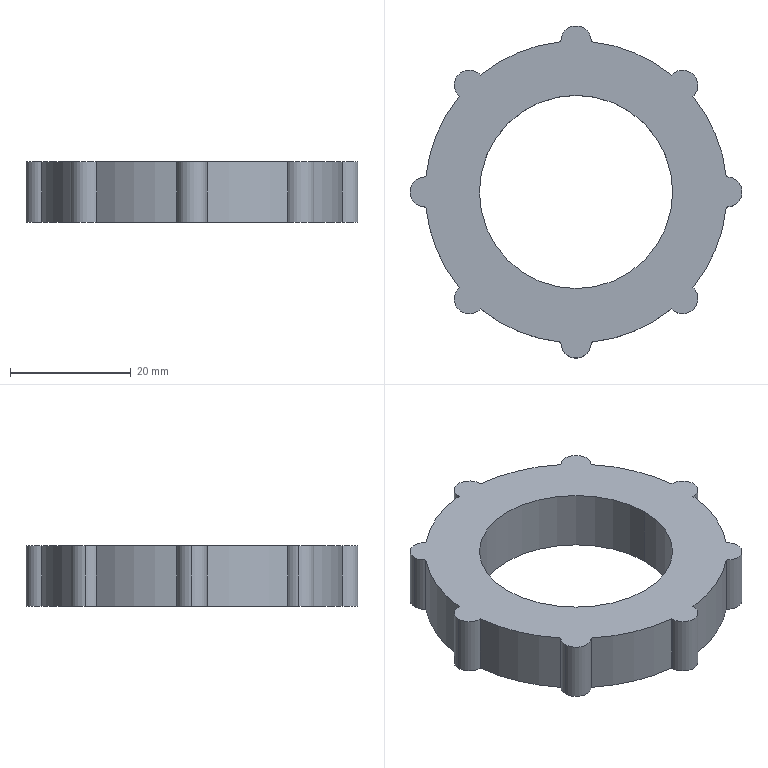Part | SolidWorks | features Extrusion 1 | 1 solid | 27 faces | box 55 x 55 x 10 mm | volume 12395 mm3 | cylinder 25 | plane 2 | commonest cylinder face diameters 5 x15 50 x8 32 x2
STEP:
#1=CARTESIAN_POINT('',(-16.,0.,10.));
#2=VERTEX_POINT('',#1);
#3=CARTESIAN_POINT('',(16.,0.,10.));
#4=VERTEX_POINT('',#3);
#5=CARTESIAN_POINT('',(0.,0.,10.));
#6=DIRECTION('',(0.,0.,1.));
#7=DIRECTION('',(1.,0.,0.));
#8=AXIS2_PLACEMENT_3D('',#5,#6,#7);
#9=CIRCLE('',#8,16.);
#10=EDGE_CURVE('',#2,#4,#9,.T.);
#11=ORIENTED_EDGE('',*,*,#10,.T.);
#12=CARTESIAN_POINT('',(16.,0.,0.));
#13=VERTEX_POINT('',#12);
#14=CARTESIAN_POINT('',(16.,0.,10.));
#15=DIRECTION('',(0.,0.,-1.));
#16=VECTOR('',#15,1000.);
#17=LINE('',#14,#16);
#18=EDGE_CURVE('',#4,#13,#17,.T.);
#19=ORIENTED_EDGE('',*,*,#18,.T.);
#20=CARTESIAN_POINT('',(-16.,0.,0.));
#21=VERTEX_POINT('',#20);
#22=CARTESIAN_POINT('',(0.,0.,0.));
#23=DIRECTION('',(0.,0.,1.));
#24=DIRECTION('',(1.,0.,0.));
#25=AXIS2_PLACEMENT_3D('',#22,#23,#24);
#26=CIRCLE('',#25,16.);
#27=EDGE_CURVE('',#21,#13,#26,.T.);
#28=ORIENTED_EDGE('',*,*,#27,.F.);
#29=CARTESIAN_POINT('',(-16.,0.,10.));
#30=DIRECTION('',(0.,0.,-1.));
#31=VECTOR('',#30,1000.);
#32=LINE('',#29,#31);
#33=EDGE_CURVE('',#2,#21,#32,.T.);
#34=ORIENTED_EDGE('',*,*,#33,.F.);
#35=EDGE_LOOP('',(#11,#19,#28,#34));
#36=FACE_OUTER_BOUND('',#35,.T.);
#37=CARTESIAN_POINT('',(0.,0.,10.));
#38=DIRECTION('',(0.,0.,-1.));
#39=DIRECTION('',(-1.,0.,0.));
#40=AXIS2_PLACEMENT_3D('',#37,#38,#39);
#41=CYLINDRICAL_SURFACE('',#40,16.);
#42=ADVANCED_FACE('',(#36),#41,.F.);
#43=CARTESIAN_POINT('',(2.5,-25.,10.));
#44=VERTEX_POINT('',#43);
#45=CARTESIAN_POINT('',(2.497,-24.875,10.));
#46=VERTEX_POINT('',#45);
#47=CARTESIAN_POINT('',(0.,-25.,10.));
#48=DIRECTION('',(0.,0.,1.));
#49=DIRECTION('',(1.,0.,0.));
#50=AXIS2_PLACEMENT_3D('',#47,#48,#49);
#51=CIRCLE('',#50,2.5);
#52=EDGE_CURVE('',#44,#46,#51,.T.);
#53=ORIENTED_EDGE('',*,*,#52,.F.);
#54=CARTESIAN_POINT('',(2.5,-25.,0.));
#55=VERTEX_POINT('',#54);
#56=CARTESIAN_POINT('',(2.5,-25.,10.));
#57=DIRECTION('',(0.,0.,-1.));
#58=VECTOR('',#57,1000.);
#59=LINE('',#56,#58);
#60=EDGE_CURVE('',#44,#55,#59,.T.);
#61=ORIENTED_EDGE('',*,*,#60,.T.);
#62=CARTESIAN_POINT('',(2.497,-24.875,0.));
#63=VERTEX_POINT('',#62);
#64=CARTESIAN_POINT('',(0.,-25.,0.));
#65=DIRECTION('',(0.,0.,1.));
#66=DIRECTION('',(1.,0.,0.));
#67=AXIS2_PLACEMENT_3D('',#64,#65,#66);
#68=CIRCLE('',#67,2.5);
#69=EDGE_CURVE('',#55,#63,#68,.T.);
#70=ORIENTED_EDGE('',*,*,#69,.T.);
#71=CARTESIAN_POINT('',(2.497,-24.875,10.));
#72=DIRECTION('',(0.,0.,-1.));
#73=VECTOR('',#72,1000.);
#74=LINE('',#71,#73);
#75=EDGE_CURVE('',#46,#63,#74,.T.);
#76=ORIENTED_EDGE('',*,*,#75,.F.);
#77=EDGE_LOOP('',(#53,#61,#70,#76));
#78=FACE_OUTER_BOUND('',#77,.T.);
#79=CARTESIAN_POINT('',(0.,-25.,10.));
#80=DIRECTION('',(0.,0.,-1.));
#81=DIRECTION('',(-1.,0.,0.));
#82=AXIS2_PLACEMENT_3D('',#79,#80,#81);
#83=CYLINDRICAL_SURFACE('',#82,2.5);
#84=ADVANCED_FACE('',(#78),#83,.T.);
#85=ORIENTED_EDGE('',*,*,#60,.F.);
#86=CARTESIAN_POINT('',(-2.5,-25.,10.));
#87=VERTEX_POINT('',#86);
#88=CARTESIAN_POINT('',(0.,-25.,10.));
#89=DIRECTION('',(0.,0.,1.));
#90=DIRECTION('',(1.,0.,0.));
#91=AXIS2_PLACEMENT_3D('',#88,#89,#90);
#92=CIRCLE('',#91,2.5);
#93=EDGE_CURVE('',#87,#44,#92,.T.);
#94=ORIENTED_EDGE('',*,*,#93,.F.);
#95=CARTESIAN_POINT('',(-2.5,-25.,0.));
#96=VERTEX_POINT('',#95);
#97=CARTESIAN_POINT('',(-2.5,-25.,10.));
#98=DIRECTION('',(0.,0.,-1.));
#99=VECTOR('',#98,1000.);
#100=LINE('',#97,#99);
#101=EDGE_CURVE('',#87,#96,#100,.T.);
#102=ORIENTED_EDGE('',*,*,#101,.T.);
#103=CARTESIAN_POINT('',(0.,-25.,0.));
#104=DIRECTION('',(0.,0.,1.));
#105=DIRECTION('',(1.,0.,0.));
#106=AXIS2_PLACEMENT_3D('',#103,#104,#105);
#107=CIRCLE('',#106,2.5);
#108=EDGE_CURVE('',#96,#55,#107,.T.);
#109=ORIENTED_EDGE('',*,*,#108,.T.);
#110=EDGE_LOOP('',(#85,#94,#102,#109));
#111=FACE_OUTER_BOUND('',#110,.T.);
#112=CARTESIAN_POINT('',(0.,-25.,10.));
#113=DIRECTION('',(0.,0.,-1.));
#114=DIRECTION('',(-1.,0.,0.));
#115=AXIS2_PLACEMENT_3D('',#112,#113,#114);
#116=CYLINDRICAL_SURFACE('',#115,2.5);
#117=ADVANCED_FACE('',(#111),#116,.T.);
#118=CARTESIAN_POINT('',(-20.178,-17.678,10.));
#119=VERTEX_POINT('',#118);
#120=CARTESIAN_POINT('',(-15.824,-19.355,10.));
#121=VERTEX_POINT('',#120);
#122=CARTESIAN_POINT('',(-17.678,-17.678,10.));
#123=DIRECTION('',(0.,0.,1.));
#124=DIRECTION('',(1.,0.,0.));
#125=AXIS2_PLACEMENT_3D('',#122,#123,#124);
#126=CIRCLE('',#125,2.5);
#127=EDGE_CURVE('',#119,#121,#126,.T.);
#128=ORIENTED_EDGE('',*,*,#127,.F.);
#129=CARTESIAN_POINT('',(-20.178,-17.678,0.));
#130=VERTEX_POINT('',#129);
#131=CARTESIAN_POINT('',(-20.178,-17.678,10.));
#132=DIRECTION('',(0.,0.,-1.));
#133=VECTOR('',#132,1000.);
#134=LINE('',#131,#133);
#135=EDGE_CURVE('',#119,#130,#134,.T.);
#136=ORIENTED_EDGE('',*,*,#135,.T.);
#137=CARTESIAN_POINT('',(-15.824,-19.355,0.));
#138=VERTEX_POINT('',#137);
#139=CARTESIAN_POINT('',(-17.678,-17.678,0.));
#140=DIRECTION('',(0.,0.,1.));
#141=DIRECTION('',(1.,0.,0.));
#142=AXIS2_PLACEMENT_3D('',#139,#140,#141);
#143=CIRCLE('',#142,2.5);
#144=EDGE_CURVE('',#130,#138,#143,.T.);
#145=ORIENTED_EDGE('',*,*,#144,.T.);
#146=CARTESIAN_POINT('',(-15.824,-19.355,10.));
#147=DIRECTION('',(0.,0.,-1.));
#148=VECTOR('',#147,1000.);
#149=LINE('',#146,#148);
#150=EDGE_CURVE('',#121,#138,#149,.T.);
#151=ORIENTED_EDGE('',*,*,#150,.F.);
#152=EDGE_LOOP('',(#128,#136,#145,#151));
#153=FACE_OUTER_BOUND('',#152,.T.);
#154=CARTESIAN_POINT('',(-17.678,-17.678,10.));
#155=DIRECTION('',(0.,0.,-1.));
#156=DIRECTION('',(-1.,0.,0.));
#157=AXIS2_PLACEMENT_3D('',#154,#155,#156);
#158=CYLINDRICAL_SURFACE('',#157,2.5);
#159=ADVANCED_FACE('',(#153),#158,.T.);
#160=CARTESIAN_POINT('',(-27.5,0.,10.));
#161=VERTEX_POINT('',#160);
#162=CARTESIAN_POINT('',(-24.875,-2.497,10.));
#163=VERTEX_POINT('',#162);
#164=CARTESIAN_POINT('',(-25.,0.,10.));
#165=DIRECTION('',(0.,0.,1.));
#166=DIRECTION('',(1.,0.,0.));
#167=AXIS2_PLACEMENT_3D('',#164,#165,#166);
#168=CIRCLE('',#167,2.5);
#169=EDGE_CURVE('',#161,#163,#168,.T.);
#170=ORIENTED_EDGE('',*,*,#169,.F.);
#171=CARTESIAN_POINT('',(-27.5,0.,0.));
#172=VERTEX_POINT('',#171);
#173=CARTESIAN_POINT('',(-27.5,0.,10.));
#174=DIRECTION('',(0.,0.,-1.));
#175=VECTOR('',#174,1000.);
#176=LINE('',#173,#175);
#177=EDGE_CURVE('',#161,#172,#176,.T.);
#178=ORIENTED_EDGE('',*,*,#177,.T.);
#179=CARTESIAN_POINT('',(-24.875,-2.497,0.));
#180=VERTEX_POINT('',#179);
#181=CARTESIAN_POINT('',(-25.,0.,0.));
#182=DIRECTION('',(0.,0.,1.));
#183=DIRECTION('',(1.,0.,0.));
#184=AXIS2_PLACEMENT_3D('',#181,#182,#183);
#185=CIRCLE('',#184,2.5);
#186=EDGE_CURVE('',#172,#180,#185,.T.);
#187=ORIENTED_EDGE('',*,*,#186,.T.);
#188=CARTESIAN_POINT('',(-24.875,-2.497,10.));
#189=DIRECTION('',(0.,0.,-1.));
#190=VECTOR('',#189,1000.);
#191=LINE('',#188,#190);
#192=EDGE_CURVE('',#163,#180,#191,.T.);
#193=ORIENTED_EDGE('',*,*,#192,.F.);
#194=EDGE_LOOP('',(#170,#178,#187,#193));
#195=FACE_OUTER_BOUND('',#194,.T.);
#196=CARTESIAN_POINT('',(-25.,0.,10.));
#197=DIRECTION('',(0.,0.,-1.));
#198=DIRECTION('',(-1.,0.,0.));
#199=AXIS2_PLACEMENT_3D('',#196,#197,#198);
#200=CYLINDRICAL_SURFACE('',#199,2.5);
#201=ADVANCED_FACE('',(#195),#200,.T.);
#202=CARTESIAN_POINT('',(-20.178,17.678,10.));
#203=VERTEX_POINT('',#202);
#204=CARTESIAN_POINT('',(-19.355,15.824,10.));
#205=VERTEX_POINT('',#204);
#206=CARTESIAN_POINT('',(-17.678,17.678,10.));
#207=DIRECTION('',(0.,0.,1.));
#208=DIRECTION('',(1.,0.,0.));
#209=AXIS2_PLACEMENT_3D('',#206,#207,#208);
#210=CIRCLE('',#209,2.5);
#211=EDGE_CURVE('',#203,#205,#210,.T.);
#212=ORIENTED_EDGE('',*,*,#211,.F.);
#213=CARTESIAN_POINT('',(-20.178,17.678,0.));
#214=VERTEX_POINT('',#213);
#215=CARTESIAN_POINT('',(-20.178,17.678,10.));
#216=DIRECTION('',(0.,0.,-1.));
#217=VECTOR('',#216,1000.);
#218=LINE('',#215,#217);
#219=EDGE_CURVE('',#203,#214,#218,.T.);
#220=ORIENTED_EDGE('',*,*,#219,.T.);
#221=CARTESIAN_POINT('',(-19.355,15.824,0.));
#222=VERTEX_POINT('',#221);
#223=CARTESIAN_POINT('',(-17.678,17.678,0.));
#224=DIRECTION('',(0.,0.,1.));
#225=DIRECTION('',(1.,0.,0.));
#226=AXIS2_PLACEMENT_3D('',#223,#224,#225);
#227=CIRCLE('',#226,2.5);
#228=EDGE_CURVE('',#214,#222,#227,.T.);
#229=ORIENTED_EDGE('',*,*,#228,.T.);
#230=CARTESIAN_POINT('',(-19.355,15.824,10.));
#231=DIRECTION('',(0.,0.,-1.));
#232=VECTOR('',#231,1000.);
#233=LINE('',#230,#232);
#234=EDGE_CURVE('',#205,#222,#233,.T.);
#235=ORIENTED_EDGE('',*,*,#234,.F.);
#236=EDGE_LOOP('',(#212,#220,#229,#235));
#237=FACE_OUTER_BOUND('',#236,.T.);
#238=CARTESIAN_POINT('',(-17.678,17.678,10.));
#239=DIRECTION('',(0.,0.,-1.));
#240=DIRECTION('',(-1.,0.,0.));
#241=AXIS2_PLACEMENT_3D('',#238,#239,#240);
#242=CYLINDRICAL_SURFACE('',#241,2.5);
#243=ADVANCED_FACE('',(#237),#242,.T.);
#244=CARTESIAN_POINT('',(2.5,25.,10.));
#245=VERTEX_POINT('',#244);
#246=CARTESIAN_POINT('',(-2.5,25.,10.));
#247=VERTEX_POINT('',#246);
#248=CARTESIAN_POINT('',(0.,25.,10.));
#249=DIRECTION('',(0.,0.,1.));
#250=DIRECTION('',(1.,0.,0.));
#251=AXIS2_PLACEMENT_3D('',#248,#249,#250);
#252=CIRCLE('',#251,2.5);
#253=EDGE_CURVE('',#245,#247,#252,.T.);
#254=ORIENTED_EDGE('',*,*,#253,.F.);
#255=CARTESIAN_POINT('',(2.5,25.,0.));
#256=VERTEX_POINT('',#255);
#257=CARTESIAN_POINT('',(2.5,25.,10.));
#258=DIRECTION('',(0.,0.,-1.));
#259=VECTOR('',#258,1000.);
#260=LINE('',#257,#259);
#261=EDGE_CURVE('',#245,#256,#260,.T.);
#262=ORIENTED_EDGE('',*,*,#261,.T.);
#263=CARTESIAN_POINT('',(-2.5,25.,0.));
#264=VERTEX_POINT('',#263);
#265=CARTESIAN_POINT('',(0.,25.,0.));
#266=DIRECTION('',(0.,0.,1.));
#267=DIRECTION('',(1.,0.,0.));
#268=AXIS2_PLACEMENT_3D('',#265,#266,#267);
#269=CIRCLE('',#268,2.5);
#270=EDGE_CURVE('',#256,#264,#269,.T.);
#271=ORIENTED_EDGE('',*,*,#270,.T.);
#272=CARTESIAN_POINT('',(-2.5,25.,10.));
#273=DIRECTION('',(0.,0.,-1.));
#274=VECTOR('',#273,1000.);
#275=LINE('',#272,#274);
#276=EDGE_CURVE('',#247,#264,#275,.T.);
#277=ORIENTED_EDGE('',*,*,#276,.F.);
#278=EDGE_LOOP('',(#254,#262,#271,#277));
#279=FACE_OUTER_BOUND('',#278,.T.);
#280=CARTESIAN_POINT('',(0.,25.,10.));
#281=DIRECTION('',(0.,0.,-1.));
#282=DIRECTION('',(-1.,0.,0.));
#283=AXIS2_PLACEMENT_3D('',#280,#281,#282);
#284=CYLINDRICAL_SURFACE('',#283,2.5);
#285=ADVANCED_FACE('',(#279),#284,.T.);
#286=CARTESIAN_POINT('',(-2.497,24.875,10.));
#287=VERTEX_POINT('',#286);
#288=CARTESIAN_POINT('',(0.,25.,10.));
#289=DIRECTION('',(0.,0.,1.));
#290=DIRECTION('',(1.,0.,0.));
#291=AXIS2_PLACEMENT_3D('',#288,#289,#290);
#292=CIRCLE('',#291,2.5);
#293=EDGE_CURVE('',#247,#287,#292,.T.);
#294=ORIENTED_EDGE('',*,*,#293,.F.);
#295=ORIENTED_EDGE('',*,*,#276,.T.);
#296=CARTESIAN_POINT('',(-2.497,24.875,0.));
#297=VERTEX_POINT('',#296);
#298=CARTESIAN_POINT('',(0.,25.,0.));
#299=DIRECTION('',(0.,0.,1.));
#300=DIRECTION('',(1.,0.,0.));
#301=AXIS2_PLACEMENT_3D('',#298,#299,#300);
#302=CIRCLE('',#301,2.5);
#303=EDGE_CURVE('',#264,#297,#302,.T.);
#304=ORIENTED_EDGE('',*,*,#303,.T.);
#305=CARTESIAN_POINT('',(-2.497,24.875,10.));
#306=DIRECTION('',(0.,0.,-1.));
#307=VECTOR('',#306,1000.);
#308=LINE('',#305,#307);
#309=EDGE_CURVE('',#287,#297,#308,.T.);
#310=ORIENTED_EDGE('',*,*,#309,.F.);
#311=EDGE_LOOP('',(#294,#295,#304,#310));
#312=FACE_OUTER_BOUND('',#311,.T.);
#313=CARTESIAN_POINT('',(0.,25.,10.));
#314=DIRECTION('',(0.,0.,-1.));
#315=DIRECTION('',(-1.,0.,0.));
#316=AXIS2_PLACEMENT_3D('',#313,#314,#315);
#317=CYLINDRICAL_SURFACE('',#316,2.5);
#318=ADVANCED_FACE('',(#312),#317,.T.);
#319=CARTESIAN_POINT('',(2.497,24.875,10.));
#320=VERTEX_POINT('',#319);
#321=CARTESIAN_POINT('',(0.,25.,10.));
#322=DIRECTION('',(0.,0.,1.));
#323=DIRECTION('',(1.,0.,0.));
#324=AXIS2_PLACEMENT_3D('',#321,#322,#323);
#325=CIRCLE('',#324,2.5);
#326=EDGE_CURVE('',#320,#245,#325,.T.);
#327=ORIENTED_EDGE('',*,*,#326,.T.);
#328=ORIENTED_EDGE('',*,*,#253,.T.);
#329=ORIENTED_EDGE('',*,*,#293,.T.);
#330=CARTESIAN_POINT('',(-15.824,19.355,10.));
#331=VERTEX_POINT('',#330);
#332=CARTESIAN_POINT('',(0.,0.,10.));
#333=DIRECTION('',(0.,0.,1.));
#334=DIRECTION('',(1.,0.,0.));
#335=AXIS2_PLACEMENT_3D('',#332,#333,#334);
#336=CIRCLE('',#335,25.);
#337=EDGE_CURVE('',#287,#331,#336,.T.);
#338=ORIENTED_EDGE('',*,*,#337,.T.);
#339=CARTESIAN_POINT('',(-17.678,17.678,10.));
#340=DIRECTION('',(0.,0.,1.));
#341=DIRECTION('',(1.,0.,0.));
#342=AXIS2_PLACEMENT_3D('',#339,#340,#341);
#343=CIRCLE('',#342,2.5);
#344=EDGE_CURVE('',#331,#203,#343,.T.);
#345=ORIENTED_EDGE('',*,*,#344,.T.);
#346=ORIENTED_EDGE('',*,*,#211,.T.);
#347=CARTESIAN_POINT('',(-24.875,2.497,10.));
#348=VERTEX_POINT('',#347);
#349=CARTESIAN_POINT('',(0.,0.,10.));
#350=DIRECTION('',(0.,0.,1.));
#351=DIRECTION('',(1.,0.,0.));
#352=AXIS2_PLACEMENT_3D('',#349,#350,#351);
#353=CIRCLE('',#352,25.);
#354=EDGE_CURVE('',#205,#348,#353,.T.);
#355=ORIENTED_EDGE('',*,*,#354,.T.);
#356=CARTESIAN_POINT('',(-25.,0.,10.));
#357=DIRECTION('',(0.,0.,1.));
#358=DIRECTION('',(1.,0.,0.));
#359=AXIS2_PLACEMENT_3D('',#356,#357,#358);
#360=CIRCLE('',#359,2.5);
#361=EDGE_CURVE('',#348,#161,#360,.T.);
#362=ORIENTED_EDGE('',*,*,#361,.T.);
#363=ORIENTED_EDGE('',*,*,#169,.T.);
#364=CARTESIAN_POINT('',(-19.355,-15.824,10.));
#365=VERTEX_POINT('',#364);
#366=CARTESIAN_POINT('',(0.,0.,10.));
#367=DIRECTION('',(0.,0.,1.));
#368=DIRECTION('',(1.,0.,0.));
#369=AXIS2_PLACEMENT_3D('',#366,#367,#368);
#370=CIRCLE('',#369,25.);
#371=EDGE_CURVE('',#163,#365,#370,.T.);
#372=ORIENTED_EDGE('',*,*,#371,.T.);
#373=CARTESIAN_POINT('',(-17.678,-17.678,10.));
#374=DIRECTION('',(0.,0.,1.));
#375=DIRECTION('',(1.,0.,0.));
#376=AXIS2_PLACEMENT_3D('',#373,#374,#375);
#377=CIRCLE('',#376,2.5);
#378=EDGE_CURVE('',#365,#119,#377,.T.);
#379=ORIENTED_EDGE('',*,*,#378,.T.);
#380=ORIENTED_EDGE('',*,*,#127,.T.);
#381=CARTESIAN_POINT('',(-2.497,-24.875,10.));
#382=VERTEX_POINT('',#381);
#383=CARTESIAN_POINT('',(0.,0.,10.));
#384=DIRECTION('',(0.,0.,1.));
#385=DIRECTION('',(1.,0.,0.));
#386=AXIS2_PLACEMENT_3D('',#383,#384,#385);
#387=CIRCLE('',#386,25.);
#388=EDGE_CURVE('',#121,#382,#387,.T.);
#389=ORIENTED_EDGE('',*,*,#388,.T.);
#390=CARTESIAN_POINT('',(0.,-25.,10.));
#391=DIRECTION('',(0.,0.,1.));
#392=DIRECTION('',(1.,0.,0.));
#393=AXIS2_PLACEMENT_3D('',#390,#391,#392);
#394=CIRCLE('',#393,2.5);
#395=EDGE_CURVE('',#382,#87,#394,.T.);
#396=ORIENTED_EDGE('',*,*,#395,.T.);
#397=ORIENTED_EDGE('',*,*,#93,.T.);
#398=ORIENTED_EDGE('',*,*,#52,.T.);
#399=CARTESIAN_POINT('',(15.824,-19.355,10.));
#400=VERTEX_POINT('',#399);
#401=CARTESIAN_POINT('',(0.,0.,10.));
#402=DIRECTION('',(0.,0.,1.));
#403=DIRECTION('',(1.,0.,0.));
#404=AXIS2_PLACEMENT_3D('',#401,#402,#403);
#405=CIRCLE('',#404,25.);
#406=EDGE_CURVE('',#46,#400,#405,.T.);
#407=ORIENTED_EDGE('',*,*,#406,.T.);
#408=CARTESIAN_POINT('',(19.355,-15.824,10.));
#409=VERTEX_POINT('',#408);
#410=CARTESIAN_POINT('',(17.678,-17.678,10.));
#411=DIRECTION('',(0.,0.,1.));
#412=DIRECTION('',(1.,0.,0.));
#413=AXIS2_PLACEMENT_3D('',#410,#411,#412);
#414=CIRCLE('',#413,2.5);
#415=EDGE_CURVE('',#400,#409,#414,.T.);
#416=ORIENTED_EDGE('',*,*,#415,.T.);
#417=CARTESIAN_POINT('',(24.875,-2.497,10.));
#418=VERTEX_POINT('',#417);
#419=CARTESIAN_POINT('',(0.,0.,10.));
#420=DIRECTION('',(0.,0.,1.));
#421=DIRECTION('',(1.,0.,0.));
#422=AXIS2_PLACEMENT_3D('',#419,#420,#421);
#423=CIRCLE('',#422,25.);
#424=EDGE_CURVE('',#409,#418,#423,.T.);
#425=ORIENTED_EDGE('',*,*,#424,.T.);
#426=CARTESIAN_POINT('',(24.875,2.497,10.));
#427=VERTEX_POINT('',#426);
#428=CARTESIAN_POINT('',(25.,0.,10.));
#429=DIRECTION('',(0.,0.,1.));
#430=DIRECTION('',(1.,0.,0.));
#431=AXIS2_PLACEMENT_3D('',#428,#429,#430);
#432=CIRCLE('',#431,2.5);
#433=EDGE_CURVE('',#418,#427,#432,.T.);
#434=ORIENTED_EDGE('',*,*,#433,.T.);
#435=CARTESIAN_POINT('',(19.355,15.824,10.));
#436=VERTEX_POINT('',#435);
#437=CARTESIAN_POINT('',(0.,0.,10.));
#438=DIRECTION('',(0.,0.,1.));
#439=DIRECTION('',(1.,0.,0.));
#440=AXIS2_PLACEMENT_3D('',#437,#438,#439);
#441=CIRCLE('',#440,25.);
#442=EDGE_CURVE('',#427,#436,#441,.T.);
#443=ORIENTED_EDGE('',*,*,#442,.T.);
#444=CARTESIAN_POINT('',(15.824,19.355,10.));
#445=VERTEX_POINT('',#444);
#446=CARTESIAN_POINT('',(17.678,17.678,10.));
#447=DIRECTION('',(0.,0.,1.));
#448=DIRECTION('',(1.,0.,0.));
#449=AXIS2_PLACEMENT_3D('',#446,#447,#448);
#450=CIRCLE('',#449,2.5);
#451=EDGE_CURVE('',#436,#445,#450,.T.);
#452=ORIENTED_EDGE('',*,*,#451,.T.);
#453=CARTESIAN_POINT('',(0.,0.,10.));
#454=DIRECTION('',(0.,0.,1.));
#455=DIRECTION('',(1.,0.,0.));
#456=AXIS2_PLACEMENT_3D('',#453,#454,#455);
#457=CIRCLE('',#456,25.);
#458=EDGE_CURVE('',#445,#320,#457,.T.);
#459=ORIENTED_EDGE('',*,*,#458,.T.);
#460=EDGE_LOOP('',(#327,#328,#329,#338,#345,#346,#355,#362,#363,#372,#379,#380,#389,#396,#397,#398,#407,#416,#425,#434,#443,#452,#459));
#461=FACE_OUTER_BOUND('',#460,.T.);
#462=ORIENTED_EDGE('',*,*,#10,.F.);
#463=CARTESIAN_POINT('',(0.,0.,10.));
#464=DIRECTION('',(0.,0.,1.));
#465=DIRECTION('',(1.,0.,0.));
#466=AXIS2_PLACEMENT_3D('',#463,#464,#465);
#467=CIRCLE('',#466,16.);
#468=EDGE_CURVE('',#4,#2,#467,.T.);
#469=ORIENTED_EDGE('',*,*,#468,.F.);
#470=EDGE_LOOP('',(#462,#469));
#471=FACE_BOUND('',#470,.T.);
#472=CARTESIAN_POINT('',(0.,12.5,10.));
#473=DIRECTION('',(0.,0.,1.));
#474=DIRECTION('',(1.,0.,0.));
#475=AXIS2_PLACEMENT_3D('',#472,#473,#474);
#476=PLANE('',#475);
#477=ADVANCED_FACE('',(#461,#471),#476,.T.);
#478=CARTESIAN_POINT('',(2.497,24.875,0.));
#479=VERTEX_POINT('',#478);
#480=CARTESIAN_POINT('',(0.,25.,0.));
#481=DIRECTION('',(0.,0.,1.));
#482=DIRECTION('',(1.,0.,0.));
#483=AXIS2_PLACEMENT_3D('',#480,#481,#482);
#484=CIRCLE('',#483,2.5);
#485=EDGE_CURVE('',#479,#256,#484,.T.);
#486=ORIENTED_EDGE('',*,*,#485,.F.);
#487=CARTESIAN_POINT('',(15.824,19.355,0.));
#488=VERTEX_POINT('',#487);
#489=CARTESIAN_POINT('',(0.,0.,0.));
#490=DIRECTION('',(0.,0.,1.));
#491=DIRECTION('',(1.,0.,0.));
#492=AXIS2_PLACEMENT_3D('',#489,#490,#491);
#493=CIRCLE('',#492,25.);
#494=EDGE_CURVE('',#488,#479,#493,.T.);
#495=ORIENTED_EDGE('',*,*,#494,.F.);
#496=CARTESIAN_POINT('',(19.355,15.824,0.));
#497=VERTEX_POINT('',#496);
#498=CARTESIAN_POINT('',(17.678,17.678,0.));
#499=DIRECTION('',(0.,0.,1.));
#500=DIRECTION('',(1.,0.,0.));
#501=AXIS2_PLACEMENT_3D('',#498,#499,#500);
#502=CIRCLE('',#501,2.5);
#503=EDGE_CURVE('',#497,#488,#502,.T.);
#504=ORIENTED_EDGE('',*,*,#503,.F.);
#505=CARTESIAN_POINT('',(24.875,2.497,0.));
#506=VERTEX_POINT('',#505);
#507=CARTESIAN_POINT('',(0.,0.,0.));
#508=DIRECTION('',(0.,0.,1.));
#509=DIRECTION('',(1.,0.,0.));
#510=AXIS2_PLACEMENT_3D('',#507,#508,#509);
#511=CIRCLE('',#510,25.);
#512=EDGE_CURVE('',#506,#497,#511,.T.);
#513=ORIENTED_EDGE('',*,*,#512,.F.);
#514=CARTESIAN_POINT('',(24.875,-2.497,0.));
#515=VERTEX_POINT('',#514);
#516=CARTESIAN_POINT('',(25.,0.,0.));
#517=DIRECTION('',(0.,0.,1.));
#518=DIRECTION('',(1.,0.,0.));
#519=AXIS2_PLACEMENT_3D('',#516,#517,#518);
#520=CIRCLE('',#519,2.5);
#521=EDGE_CURVE('',#515,#506,#520,.T.);
#522=ORIENTED_EDGE('',*,*,#521,.F.);
#523=CARTESIAN_POINT('',(19.355,-15.824,0.));
#524=VERTEX_POINT('',#523);
#525=CARTESIAN_POINT('',(0.,0.,0.));
#526=DIRECTION('',(0.,0.,1.));
#527=DIRECTION('',(1.,0.,0.));
#528=AXIS2_PLACEMENT_3D('',#525,#526,#527);
#529=CIRCLE('',#528,25.);
#530=EDGE_CURVE('',#524,#515,#529,.T.);
#531=ORIENTED_EDGE('',*,*,#530,.F.);
#532=CARTESIAN_POINT('',(15.824,-19.355,0.));
#533=VERTEX_POINT('',#532);
#534=CARTESIAN_POINT('',(17.678,-17.678,0.));
#535=DIRECTION('',(0.,0.,1.));
#536=DIRECTION('',(1.,0.,0.));
#537=AXIS2_PLACEMENT_3D('',#534,#535,#536);
#538=CIRCLE('',#537,2.5);
#539=EDGE_CURVE('',#533,#524,#538,.T.);
#540=ORIENTED_EDGE('',*,*,#539,.F.);
#541=CARTESIAN_POINT('',(0.,0.,0.));
#542=DIRECTION('',(0.,0.,1.));
#543=DIRECTION('',(1.,0.,0.));
#544=AXIS2_PLACEMENT_3D('',#541,#542,#543);
#545=CIRCLE('',#544,25.);
#546=EDGE_CURVE('',#63,#533,#545,.T.);
#547=ORIENTED_EDGE('',*,*,#546,.F.);
#548=ORIENTED_EDGE('',*,*,#69,.F.);
#549=ORIENTED_EDGE('',*,*,#108,.F.);
#550=CARTESIAN_POINT('',(-2.497,-24.875,0.));
#551=VERTEX_POINT('',#550);
#552=CARTESIAN_POINT('',(0.,-25.,0.));
#553=DIRECTION('',(0.,0.,1.));
#554=DIRECTION('',(1.,0.,0.));
#555=AXIS2_PLACEMENT_3D('',#552,#553,#554);
#556=CIRCLE('',#555,2.5);
#557=EDGE_CURVE('',#551,#96,#556,.T.);
#558=ORIENTED_EDGE('',*,*,#557,.F.);
#559=CARTESIAN_POINT('',(0.,0.,0.));
#560=DIRECTION('',(0.,0.,1.));
#561=DIRECTION('',(1.,0.,0.));
#562=AXIS2_PLACEMENT_3D('',#559,#560,#561);
#563=CIRCLE('',#562,25.);
#564=EDGE_CURVE('',#138,#551,#563,.T.);
#565=ORIENTED_EDGE('',*,*,#564,.F.);
#566=ORIENTED_EDGE('',*,*,#144,.F.);
#567=CARTESIAN_POINT('',(-19.355,-15.824,0.));
#568=VERTEX_POINT('',#567);
#569=CARTESIAN_POINT('',(-17.678,-17.678,0.));
#570=DIRECTION('',(0.,0.,1.));
#571=DIRECTION('',(1.,0.,0.));
#572=AXIS2_PLACEMENT_3D('',#569,#570,#571);
#573=CIRCLE('',#572,2.5);
#574=EDGE_CURVE('',#568,#130,#573,.T.);
#575=ORIENTED_EDGE('',*,*,#574,.F.);
#576=CARTESIAN_POINT('',(0.,0.,0.));
#577=DIRECTION('',(0.,0.,1.));
#578=DIRECTION('',(1.,0.,0.));
#579=AXIS2_PLACEMENT_3D('',#576,#577,#578);
#580=CIRCLE('',#579,25.);
#581=EDGE_CURVE('',#180,#568,#580,.T.);
#582=ORIENTED_EDGE('',*,*,#581,.F.);
#583=ORIENTED_EDGE('',*,*,#186,.F.);
#584=CARTESIAN_POINT('',(-24.875,2.497,0.));
#585=VERTEX_POINT('',#584);
#586=CARTESIAN_POINT('',(-25.,0.,0.));
#587=DIRECTION('',(0.,0.,1.));
#588=DIRECTION('',(1.,0.,0.));
#589=AXIS2_PLACEMENT_3D('',#586,#587,#588);
#590=CIRCLE('',#589,2.5);
#591=EDGE_CURVE('',#585,#172,#590,.T.);
#592=ORIENTED_EDGE('',*,*,#591,.F.);
#593=CARTESIAN_POINT('',(0.,0.,0.));
#594=DIRECTION('',(0.,0.,1.));
#595=DIRECTION('',(1.,0.,0.));
#596=AXIS2_PLACEMENT_3D('',#593,#594,#595);
#597=CIRCLE('',#596,25.);
#598=EDGE_CURVE('',#222,#585,#597,.T.);
#599=ORIENTED_EDGE('',*,*,#598,.F.);
#600=ORIENTED_EDGE('',*,*,#228,.F.);
#601=CARTESIAN_POINT('',(-15.824,19.355,0.));
#602=VERTEX_POINT('',#601);
#603=CARTESIAN_POINT('',(-17.678,17.678,0.));
#604=DIRECTION('',(0.,0.,1.));
#605=DIRECTION('',(1.,0.,0.));
#606=AXIS2_PLACEMENT_3D('',#603,#604,#605);
#607=CIRCLE('',#606,2.5);
#608=EDGE_CURVE('',#602,#214,#607,.T.);
#609=ORIENTED_EDGE('',*,*,#608,.F.);
#610=CARTESIAN_POINT('',(0.,0.,0.));
#611=DIRECTION('',(0.,0.,1.));
#612=DIRECTION('',(1.,0.,0.));
#613=AXIS2_PLACEMENT_3D('',#610,#611,#612);
#614=CIRCLE('',#613,25.);
#615=EDGE_CURVE('',#297,#602,#614,.T.);
#616=ORIENTED_EDGE('',*,*,#615,.F.);
#617=ORIENTED_EDGE('',*,*,#303,.F.);
#618=ORIENTED_EDGE('',*,*,#270,.F.);
#619=EDGE_LOOP('',(#486,#495,#504,#513,#522,#531,#540,#547,#548,#549,#558,#565,#566,#575,#582,#583,#592,#599,#600,#609,#616,#617,#618));
#620=FACE_OUTER_BOUND('',#619,.T.);
#621=ORIENTED_EDGE('',*,*,#27,.T.);
#622=CARTESIAN_POINT('',(0.,0.,0.));
#623=DIRECTION('',(0.,0.,1.));
#624=DIRECTION('',(1.,0.,0.));
#625=AXIS2_PLACEMENT_3D('',#622,#623,#624);
#626=CIRCLE('',#625,16.);
#627=EDGE_CURVE('',#13,#21,#626,.T.);
#628=ORIENTED_EDGE('',*,*,#627,.T.);
#629=EDGE_LOOP('',(#621,#628));
#630=FACE_BOUND('',#629,.T.);
#631=CARTESIAN_POINT('',(0.,12.5,0.));
#632=DIRECTION('',(0.,0.,1.));
#633=DIRECTION('',(1.,0.,0.));
#634=AXIS2_PLACEMENT_3D('',#631,#632,#633);
#635=PLANE('',#634);
#636=ADVANCED_FACE('',(#620,#630),#635,.F.);
#637=ORIENTED_EDGE('',*,*,#261,.F.);
#638=ORIENTED_EDGE('',*,*,#326,.F.);
#639=CARTESIAN_POINT('',(2.497,24.875,10.));
#640=DIRECTION('',(0.,0.,-1.));
#641=VECTOR('',#640,1000.);
#642=LINE('',#639,#641);
#643=EDGE_CURVE('',#320,#479,#642,.T.);
#644=ORIENTED_EDGE('',*,*,#643,.T.);
#645=ORIENTED_EDGE('',*,*,#485,.T.);
#646=EDGE_LOOP('',(#637,#638,#644,#645));
#647=FACE_OUTER_BOUND('',#646,.T.);
#648=CARTESIAN_POINT('',(0.,25.,10.));
#649=DIRECTION('',(0.,0.,-1.));
#650=DIRECTION('',(-1.,0.,0.));
#651=AXIS2_PLACEMENT_3D('',#648,#649,#650);
#652=CYLINDRICAL_SURFACE('',#651,2.5);
#653=ADVANCED_FACE('',(#647),#652,.T.);
#654=ORIENTED_EDGE('',*,*,#615,.T.);
#655=CARTESIAN_POINT('',(-15.824,19.355,10.));
#656=DIRECTION('',(0.,0.,-1.));
#657=VECTOR('',#656,1000.);
#658=LINE('',#655,#657);
#659=EDGE_CURVE('',#331,#602,#658,.T.);
#660=ORIENTED_EDGE('',*,*,#659,.F.);
#661=ORIENTED_EDGE('',*,*,#337,.F.);
#662=ORIENTED_EDGE('',*,*,#309,.T.);
#663=EDGE_LOOP('',(#654,#660,#661,#662));
#664=FACE_OUTER_BOUND('',#663,.T.);
#665=CARTESIAN_POINT('',(0.,0.,10.));
#666=DIRECTION('',(0.,0.,-1.));
#667=DIRECTION('',(-1.,0.,0.));
#668=AXIS2_PLACEMENT_3D('',#665,#666,#667);
#669=CYLINDRICAL_SURFACE('',#668,25.);
#670=ADVANCED_FACE('',(#664),#669,.T.);
#671=ORIENTED_EDGE('',*,*,#219,.F.);
#672=ORIENTED_EDGE('',*,*,#344,.F.);
#673=ORIENTED_EDGE('',*,*,#659,.T.);
#674=ORIENTED_EDGE('',*,*,#608,.T.);
#675=EDGE_LOOP('',(#671,#672,#673,#674));
#676=FACE_OUTER_BOUND('',#675,.T.);
#677=CARTESIAN_POINT('',(-17.678,17.678,10.));
#678=DIRECTION('',(0.,0.,-1.));
#679=DIRECTION('',(-1.,0.,0.));
#680=AXIS2_PLACEMENT_3D('',#677,#678,#679);
#681=CYLINDRICAL_SURFACE('',#680,2.5);
#682=ADVANCED_FACE('',(#676),#681,.T.);
#683=ORIENTED_EDGE('',*,*,#598,.T.);
#684=CARTESIAN_POINT('',(-24.875,2.497,10.));
#685=DIRECTION('',(0.,0.,-1.));
#686=VECTOR('',#685,1000.);
#687=LINE('',#684,#686);
#688=EDGE_CURVE('',#348,#585,#687,.T.);
#689=ORIENTED_EDGE('',*,*,#688,.F.);
#690=ORIENTED_EDGE('',*,*,#354,.F.);
#691=ORIENTED_EDGE('',*,*,#234,.T.);
#692=EDGE_LOOP('',(#683,#689,#690,#691));
#693=FACE_OUTER_BOUND('',#692,.T.);
#694=CARTESIAN_POINT('',(0.,0.,10.));
#695=DIRECTION('',(0.,0.,-1.));
#696=DIRECTION('',(-1.,0.,0.));
#697=AXIS2_PLACEMENT_3D('',#694,#695,#696);
#698=CYLINDRICAL_SURFACE('',#697,25.);
#699=ADVANCED_FACE('',(#693),#698,.T.);
#700=ORIENTED_EDGE('',*,*,#177,.F.);
#701=ORIENTED_EDGE('',*,*,#361,.F.);
#702=ORIENTED_EDGE('',*,*,#688,.T.);
#703=ORIENTED_EDGE('',*,*,#591,.T.);
#704=EDGE_LOOP('',(#700,#701,#702,#703));
#705=FACE_OUTER_BOUND('',#704,.T.);
#706=CARTESIAN_POINT('',(-25.,0.,10.));
#707=DIRECTION('',(0.,0.,-1.));
#708=DIRECTION('',(-1.,0.,0.));
#709=AXIS2_PLACEMENT_3D('',#706,#707,#708);
#710=CYLINDRICAL_SURFACE('',#709,2.5);
#711=ADVANCED_FACE('',(#705),#710,.T.);
#712=ORIENTED_EDGE('',*,*,#581,.T.);
#713=CARTESIAN_POINT('',(-19.355,-15.824,10.));
#714=DIRECTION('',(0.,0.,-1.));
#715=VECTOR('',#714,1000.);
#716=LINE('',#713,#715);
#717=EDGE_CURVE('',#365,#568,#716,.T.);
#718=ORIENTED_EDGE('',*,*,#717,.F.);
#719=ORIENTED_EDGE('',*,*,#371,.F.);
#720=ORIENTED_EDGE('',*,*,#192,.T.);
#721=EDGE_LOOP('',(#712,#718,#719,#720));
#722=FACE_OUTER_BOUND('',#721,.T.);
#723=CARTESIAN_POINT('',(0.,0.,10.));
#724=DIRECTION('',(0.,0.,-1.));
#725=DIRECTION('',(-1.,0.,0.));
#726=AXIS2_PLACEMENT_3D('',#723,#724,#725);
#727=CYLINDRICAL_SURFACE('',#726,25.);
#728=ADVANCED_FACE('',(#722),#727,.T.);
#729=ORIENTED_EDGE('',*,*,#135,.F.);
#730=ORIENTED_EDGE('',*,*,#378,.F.);
#731=ORIENTED_EDGE('',*,*,#717,.T.);
#732=ORIENTED_EDGE('',*,*,#574,.T.);
#733=EDGE_LOOP('',(#729,#730,#731,#732));
#734=FACE_OUTER_BOUND('',#733,.T.);
#735=CARTESIAN_POINT('',(-17.678,-17.678,10.));
#736=DIRECTION('',(0.,0.,-1.));
#737=DIRECTION('',(-1.,0.,0.));
#738=AXIS2_PLACEMENT_3D('',#735,#736,#737);
#739=CYLINDRICAL_SURFACE('',#738,2.5);
#740=ADVANCED_FACE('',(#734),#739,.T.);
#741=ORIENTED_EDGE('',*,*,#564,.T.);
#742=CARTESIAN_POINT('',(-2.497,-24.875,10.));
#743=DIRECTION('',(0.,0.,-1.));
#744=VECTOR('',#743,1000.);
#745=LINE('',#742,#744);
#746=EDGE_CURVE('',#382,#551,#745,.T.);
#747=ORIENTED_EDGE('',*,*,#746,.F.);
#748=ORIENTED_EDGE('',*,*,#388,.F.);
#749=ORIENTED_EDGE('',*,*,#150,.T.);
#750=EDGE_LOOP('',(#741,#747,#748,#749));
#751=FACE_OUTER_BOUND('',#750,.T.);
#752=CARTESIAN_POINT('',(0.,0.,10.));
#753=DIRECTION('',(0.,0.,-1.));
#754=DIRECTION('',(-1.,0.,0.));
#755=AXIS2_PLACEMENT_3D('',#752,#753,#754);
#756=CYLINDRICAL_SURFACE('',#755,25.);
#757=ADVANCED_FACE('',(#751),#756,.T.);
#758=ORIENTED_EDGE('',*,*,#101,.F.);
#759=ORIENTED_EDGE('',*,*,#395,.F.);
#760=ORIENTED_EDGE('',*,*,#746,.T.);
#761=ORIENTED_EDGE('',*,*,#557,.T.);
#762=EDGE_LOOP('',(#758,#759,#760,#761));
#763=FACE_OUTER_BOUND('',#762,.T.);
#764=CARTESIAN_POINT('',(0.,-25.,10.));
#765=DIRECTION('',(0.,0.,-1.));
#766=DIRECTION('',(-1.,0.,0.));
#767=AXIS2_PLACEMENT_3D('',#764,#765,#766);
#768=CYLINDRICAL_SURFACE('',#767,2.5);
#769=ADVANCED_FACE('',(#763),#768,.T.);
#770=ORIENTED_EDGE('',*,*,#546,.T.);
#771=CARTESIAN_POINT('',(15.824,-19.355,10.));
#772=DIRECTION('',(0.,0.,-1.));
#773=VECTOR('',#772,1000.);
#774=LINE('',#771,#773);
#775=EDGE_CURVE('',#400,#533,#774,.T.);
#776=ORIENTED_EDGE('',*,*,#775,.F.);
#777=ORIENTED_EDGE('',*,*,#406,.F.);
#778=ORIENTED_EDGE('',*,*,#75,.T.);
#779=EDGE_LOOP('',(#770,#776,#777,#778));
#780=FACE_OUTER_BOUND('',#779,.T.);
#781=CARTESIAN_POINT('',(0.,0.,10.));
#782=DIRECTION('',(0.,0.,-1.));
#783=DIRECTION('',(-1.,0.,0.));
#784=AXIS2_PLACEMENT_3D('',#781,#782,#783);
#785=CYLINDRICAL_SURFACE('',#784,25.);
#786=ADVANCED_FACE('',(#780),#785,.T.);
#787=ORIENTED_EDGE('',*,*,#539,.T.);
#788=CARTESIAN_POINT('',(19.355,-15.824,10.));
#789=DIRECTION('',(0.,0.,-1.));
#790=VECTOR('',#789,1000.);
#791=LINE('',#788,#790);
#792=EDGE_CURVE('',#409,#524,#791,.T.);
#793=ORIENTED_EDGE('',*,*,#792,.F.);
#794=ORIENTED_EDGE('',*,*,#415,.F.);
#795=ORIENTED_EDGE('',*,*,#775,.T.);
#796=EDGE_LOOP('',(#787,#793,#794,#795));
#797=FACE_OUTER_BOUND('',#796,.T.);
#798=CARTESIAN_POINT('',(17.678,-17.678,10.));
#799=DIRECTION('',(0.,0.,-1.));
#800=DIRECTION('',(-1.,0.,0.));
#801=AXIS2_PLACEMENT_3D('',#798,#799,#800);
#802=CYLINDRICAL_SURFACE('',#801,2.5);
#803=ADVANCED_FACE('',(#797),#802,.T.);
#804=ORIENTED_EDGE('',*,*,#530,.T.);
#805=CARTESIAN_POINT('',(24.875,-2.497,10.));
#806=DIRECTION('',(0.,0.,-1.));
#807=VECTOR('',#806,1000.);
#808=LINE('',#805,#807);
#809=EDGE_CURVE('',#418,#515,#808,.T.);
#810=ORIENTED_EDGE('',*,*,#809,.F.);
#811=ORIENTED_EDGE('',*,*,#424,.F.);
#812=ORIENTED_EDGE('',*,*,#792,.T.);
#813=EDGE_LOOP('',(#804,#810,#811,#812));
#814=FACE_OUTER_BOUND('',#813,.T.);
#815=CARTESIAN_POINT('',(0.,0.,10.));
#816=DIRECTION('',(0.,0.,-1.));
#817=DIRECTION('',(-1.,0.,0.));
#818=AXIS2_PLACEMENT_3D('',#815,#816,#817);
#819=CYLINDRICAL_SURFACE('',#818,25.);
#820=ADVANCED_FACE('',(#814),#819,.T.);
#821=ORIENTED_EDGE('',*,*,#521,.T.);
#822=CARTESIAN_POINT('',(24.875,2.497,10.));
#823=DIRECTION('',(0.,0.,-1.));
#824=VECTOR('',#823,1000.);
#825=LINE('',#822,#824);
#826=EDGE_CURVE('',#427,#506,#825,.T.);
#827=ORIENTED_EDGE('',*,*,#826,.F.);
#828=ORIENTED_EDGE('',*,*,#433,.F.);
#829=ORIENTED_EDGE('',*,*,#809,.T.);
#830=EDGE_LOOP('',(#821,#827,#828,#829));
#831=FACE_OUTER_BOUND('',#830,.T.);
#832=CARTESIAN_POINT('',(25.,0.,10.));
#833=DIRECTION('',(0.,0.,-1.));
#834=DIRECTION('',(-1.,0.,0.));
#835=AXIS2_PLACEMENT_3D('',#832,#833,#834);
#836=CYLINDRICAL_SURFACE('',#835,2.5);
#837=ADVANCED_FACE('',(#831),#836,.T.);
#838=ORIENTED_EDGE('',*,*,#512,.T.);
#839=CARTESIAN_POINT('',(19.355,15.824,10.));
#840=DIRECTION('',(0.,0.,-1.));
#841=VECTOR('',#840,1000.);
#842=LINE('',#839,#841);
#843=EDGE_CURVE('',#436,#497,#842,.T.);
#844=ORIENTED_EDGE('',*,*,#843,.F.);
#845=ORIENTED_EDGE('',*,*,#442,.F.);
#846=ORIENTED_EDGE('',*,*,#826,.T.);
#847=EDGE_LOOP('',(#838,#844,#845,#846));
#848=FACE_OUTER_BOUND('',#847,.T.);
#849=CARTESIAN_POINT('',(0.,0.,10.));
#850=DIRECTION('',(0.,0.,-1.));
#851=DIRECTION('',(-1.,0.,0.));
#852=AXIS2_PLACEMENT_3D('',#849,#850,#851);
#853=CYLINDRICAL_SURFACE('',#852,25.);
#854=ADVANCED_FACE('',(#848),#853,.T.);
#855=ORIENTED_EDGE('',*,*,#503,.T.);
#856=CARTESIAN_POINT('',(15.824,19.355,10.));
#857=DIRECTION('',(0.,0.,-1.));
#858=VECTOR('',#857,1000.);
#859=LINE('',#856,#858);
#860=EDGE_CURVE('',#445,#488,#859,.T.);
#861=ORIENTED_EDGE('',*,*,#860,.F.);
#862=ORIENTED_EDGE('',*,*,#451,.F.);
#863=ORIENTED_EDGE('',*,*,#843,.T.);
#864=EDGE_LOOP('',(#855,#861,#862,#863));
#865=FACE_OUTER_BOUND('',#864,.T.);
#866=CARTESIAN_POINT('',(17.678,17.678,10.));
#867=DIRECTION('',(0.,0.,-1.));
#868=DIRECTION('',(-1.,0.,0.));
#869=AXIS2_PLACEMENT_3D('',#866,#867,#868);
#870=CYLINDRICAL_SURFACE('',#869,2.5);
#871=ADVANCED_FACE('',(#865),#870,.T.);
#872=ORIENTED_EDGE('',*,*,#494,.T.);
#873=ORIENTED_EDGE('',*,*,#643,.F.);
#874=ORIENTED_EDGE('',*,*,#458,.F.);
#875=ORIENTED_EDGE('',*,*,#860,.T.);
#876=EDGE_LOOP('',(#872,#873,#874,#875));
#877=FACE_OUTER_BOUND('',#876,.T.);
#878=CARTESIAN_POINT('',(0.,0.,10.));
#879=DIRECTION('',(0.,0.,-1.));
#880=DIRECTION('',(-1.,0.,0.));
#881=AXIS2_PLACEMENT_3D('',#878,#879,#880);
#882=CYLINDRICAL_SURFACE('',#881,25.);
#883=ADVANCED_FACE('',(#877),#882,.T.);
#884=ORIENTED_EDGE('',*,*,#18,.F.);
#885=ORIENTED_EDGE('',*,*,#468,.T.);
#886=ORIENTED_EDGE('',*,*,#33,.T.);
#887=ORIENTED_EDGE('',*,*,#627,.F.);
#888=EDGE_LOOP('',(#884,#885,#886,#887));
#889=FACE_OUTER_BOUND('',#888,.T.);
#890=CARTESIAN_POINT('',(0.,0.,10.));
#891=DIRECTION('',(0.,0.,-1.));
#892=DIRECTION('',(-1.,0.,0.));
#893=AXIS2_PLACEMENT_3D('',#890,#891,#892);
#894=CYLINDRICAL_SURFACE('',#893,16.);
#895=ADVANCED_FACE('',(#889),#894,.F.);
#896=CLOSED_SHELL('',(#42,#84,#117,#159,#201,#243,#285,#318,#477,#636,#653,#670,#682,#699,#711,#728,#740,#757,#769,#786,#803,#820,#837,#854,#871,#883,#895));
#897=MANIFOLD_SOLID_BREP('',#896);
#898=CARTESIAN_POINT('',(0.,0.,0.));
#899=DIRECTION('',(0.,0.,1.));
#900=DIRECTION('',(1.,0.,0.));
#901=AXIS2_PLACEMENT_3D('',#898,#899,#900);
#902=(LENGTH_UNIT()NAMED_UNIT(*)SI_UNIT(.MILLI.,.METRE.));
#903=UNCERTAINTY_MEASURE_WITH_UNIT(LENGTH_MEASURE(0.00001),#902,'','');
#904=(NAMED_UNIT(*)PLANE_ANGLE_UNIT()SI_UNIT($,.RADIAN.));
#905=(NAMED_UNIT(*)SI_UNIT($,.STERADIAN.)SOLID_ANGLE_UNIT());
#906=(GEOMETRIC_REPRESENTATION_CONTEXT(3)GLOBAL_UNCERTAINTY_ASSIGNED_CONTEXT((#903))GLOBAL_UNIT_ASSIGNED_CONTEXT((#902,#904,#905))REPRESENTATION_CONTEXT('',''));
#907=ADVANCED_BREP_SHAPE_REPRESENTATION('',(#897,#901),#906);